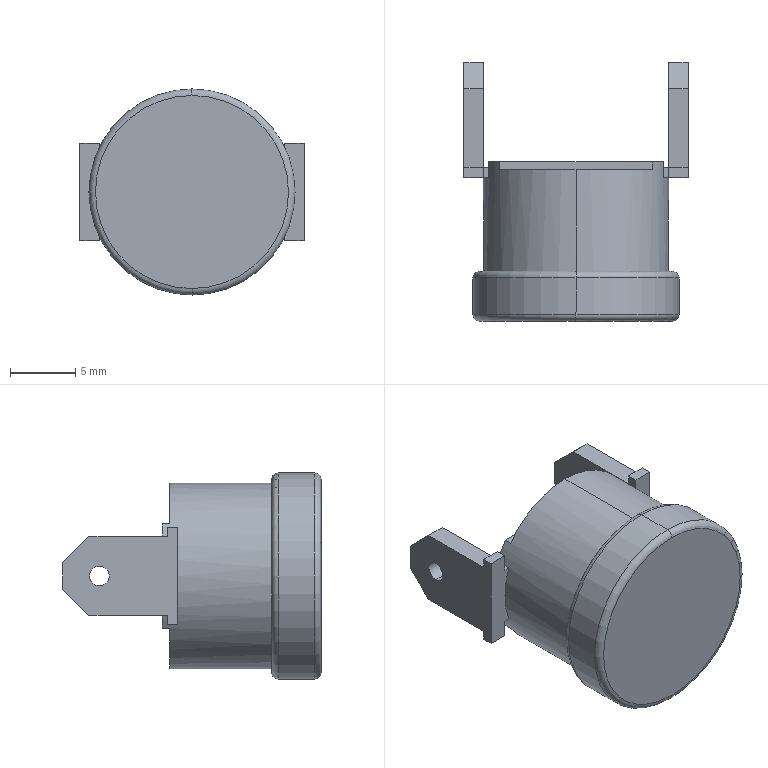Part | STEP file | WENKONGQI_16_1 | 1 solid | 55 faces | box 17.2 x 19.8 x 15.8 mm | volume 2165 mm3 | plane 43 | cylinder 8 | torus 4 | commonest cylinder face diameters 1.5 x4 14.2 x2 15.8 x2